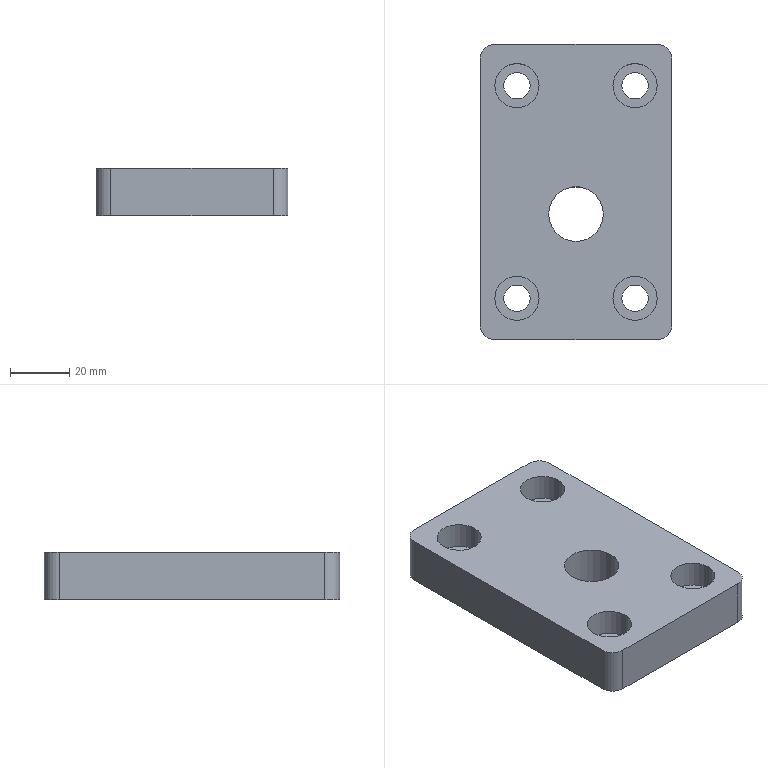Part | NX | features BREP 1 | 1 solid | 32 faces | box 65 x 100 x 16 mm | volume 91213 mm3 | cylinder 22 | plane 10 | commonest cylinder face diameters 9 x8 15 x8 10 x4 18.5 x2
STEP:
#1=CARTESIAN_POINT('',(-9.25,-7.5,0.));
#2=VERTEX_POINT('',#1);
#3=CARTESIAN_POINT('',(9.25,-7.5,0.));
#4=VERTEX_POINT('',#3);
#5=CARTESIAN_POINT('',(0.,-7.5,0.));
#6=DIRECTION('',(0.,0.,1.));
#7=DIRECTION('',(1.,0.,0.));
#8=AXIS2_PLACEMENT_3D('',#5,#6,#7);
#9=CIRCLE('',#8,9.25);
#10=EDGE_CURVE('',#2,#4,#9,.T.);
#11=ORIENTED_EDGE('',*,*,#10,.F.);
#12=CARTESIAN_POINT('',(-9.25,-7.5,16.));
#13=VERTEX_POINT('',#12);
#14=CARTESIAN_POINT('',(-9.25,-7.5,16.));
#15=DIRECTION('',(0.,0.,1.));
#16=VECTOR('',#15,1000.);
#17=LINE('',#14,#16);
#18=EDGE_CURVE('',#13,#2,#17,.F.);
#19=ORIENTED_EDGE('',*,*,#18,.F.);
#20=CARTESIAN_POINT('',(9.25,-7.5,16.));
#21=VERTEX_POINT('',#20);
#22=CARTESIAN_POINT('',(0.,-7.5,16.));
#23=DIRECTION('',(0.,0.,1.));
#24=DIRECTION('',(1.,0.,0.));
#25=AXIS2_PLACEMENT_3D('',#22,#23,#24);
#26=CIRCLE('',#25,9.25);
#27=EDGE_CURVE('',#13,#21,#26,.T.);
#28=ORIENTED_EDGE('',*,*,#27,.T.);
#29=CARTESIAN_POINT('',(9.25,-7.5,16.));
#30=DIRECTION('',(0.,0.,1.));
#31=VECTOR('',#30,1000.);
#32=LINE('',#29,#31);
#33=EDGE_CURVE('',#21,#4,#32,.F.);
#34=ORIENTED_EDGE('',*,*,#33,.T.);
#35=EDGE_LOOP('',(#11,#19,#28,#34));
#36=FACE_BOUND('',#35,.T.);
#37=CARTESIAN_POINT('',(0.,-7.5,16.));
#38=DIRECTION('',(0.,0.,1.));
#39=DIRECTION('',(1.,0.,0.));
#40=AXIS2_PLACEMENT_3D('',#37,#38,#39);
#41=CYLINDRICAL_SURFACE('',#40,9.25);
#42=ADVANCED_FACE('',(#36),#41,.F.);
#43=CARTESIAN_POINT('',(-27.5,36.,7.));
#44=VERTEX_POINT('',#43);
#45=CARTESIAN_POINT('',(-12.5,36.,7.));
#46=VERTEX_POINT('',#45);
#47=CARTESIAN_POINT('',(-20.,36.,7.));
#48=DIRECTION('',(0.,0.,1.));
#49=DIRECTION('',(1.,0.,0.));
#50=AXIS2_PLACEMENT_3D('',#47,#48,#49);
#51=CIRCLE('',#50,7.5);
#52=EDGE_CURVE('',#44,#46,#51,.T.);
#53=ORIENTED_EDGE('',*,*,#52,.F.);
#54=CARTESIAN_POINT('',(-27.5,36.,16.));
#55=VERTEX_POINT('',#54);
#56=CARTESIAN_POINT('',(-27.5,36.,16.));
#57=DIRECTION('',(0.,0.,1.));
#58=VECTOR('',#57,1000.);
#59=LINE('',#56,#58);
#60=EDGE_CURVE('',#55,#44,#59,.F.);
#61=ORIENTED_EDGE('',*,*,#60,.F.);
#62=CARTESIAN_POINT('',(-12.5,36.,16.));
#63=VERTEX_POINT('',#62);
#64=CARTESIAN_POINT('',(-20.,36.,16.));
#65=DIRECTION('',(0.,0.,1.));
#66=DIRECTION('',(1.,0.,0.));
#67=AXIS2_PLACEMENT_3D('',#64,#65,#66);
#68=CIRCLE('',#67,7.5);
#69=EDGE_CURVE('',#55,#63,#68,.T.);
#70=ORIENTED_EDGE('',*,*,#69,.T.);
#71=CARTESIAN_POINT('',(-12.5,36.,16.));
#72=DIRECTION('',(0.,0.,1.));
#73=VECTOR('',#72,1000.);
#74=LINE('',#71,#73);
#75=EDGE_CURVE('',#63,#46,#74,.F.);
#76=ORIENTED_EDGE('',*,*,#75,.T.);
#77=EDGE_LOOP('',(#53,#61,#70,#76));
#78=FACE_BOUND('',#77,.T.);
#79=CARTESIAN_POINT('',(-20.,36.,16.));
#80=DIRECTION('',(0.,0.,1.));
#81=DIRECTION('',(1.,0.,0.));
#82=AXIS2_PLACEMENT_3D('',#79,#80,#81);
#83=CYLINDRICAL_SURFACE('',#82,7.5);
#84=ADVANCED_FACE('',(#78),#83,.F.);
#85=CARTESIAN_POINT('',(-24.5,36.,0.));
#86=VERTEX_POINT('',#85);
#87=CARTESIAN_POINT('',(-15.5,36.,0.));
#88=VERTEX_POINT('',#87);
#89=CARTESIAN_POINT('',(-20.,36.,0.));
#90=DIRECTION('',(0.,0.,1.));
#91=DIRECTION('',(1.,0.,0.));
#92=AXIS2_PLACEMENT_3D('',#89,#90,#91);
#93=CIRCLE('',#92,4.5);
#94=EDGE_CURVE('',#86,#88,#93,.T.);
#95=ORIENTED_EDGE('',*,*,#94,.F.);
#96=CARTESIAN_POINT('',(-24.5,36.,7.));
#97=VERTEX_POINT('',#96);
#98=CARTESIAN_POINT('',(-24.5,36.,16.));
#99=DIRECTION('',(0.,0.,1.));
#100=VECTOR('',#99,1000.);
#101=LINE('',#98,#100);
#102=EDGE_CURVE('',#97,#86,#101,.F.);
#103=ORIENTED_EDGE('',*,*,#102,.F.);
#104=CARTESIAN_POINT('',(-15.5,36.,7.));
#105=VERTEX_POINT('',#104);
#106=CARTESIAN_POINT('',(-20.,36.,7.));
#107=DIRECTION('',(0.,0.,1.));
#108=DIRECTION('',(1.,0.,0.));
#109=AXIS2_PLACEMENT_3D('',#106,#107,#108);
#110=CIRCLE('',#109,4.5);
#111=EDGE_CURVE('',#97,#105,#110,.T.);
#112=ORIENTED_EDGE('',*,*,#111,.T.);
#113=CARTESIAN_POINT('',(-15.5,36.,16.));
#114=DIRECTION('',(0.,0.,1.));
#115=VECTOR('',#114,1000.);
#116=LINE('',#113,#115);
#117=EDGE_CURVE('',#105,#88,#116,.F.);
#118=ORIENTED_EDGE('',*,*,#117,.T.);
#119=EDGE_LOOP('',(#95,#103,#112,#118));
#120=FACE_BOUND('',#119,.T.);
#121=CARTESIAN_POINT('',(-20.,36.,16.));
#122=DIRECTION('',(0.,0.,1.));
#123=DIRECTION('',(1.,0.,0.));
#124=AXIS2_PLACEMENT_3D('',#121,#122,#123);
#125=CYLINDRICAL_SURFACE('',#124,4.5);
#126=ADVANCED_FACE('',(#120),#125,.F.);
#127=CARTESIAN_POINT('',(12.5,36.,7.));
#128=VERTEX_POINT('',#127);
#129=CARTESIAN_POINT('',(27.5,36.,7.));
#130=VERTEX_POINT('',#129);
#131=CARTESIAN_POINT('',(20.,36.,7.));
#132=DIRECTION('',(0.,0.,1.));
#133=DIRECTION('',(1.,0.,0.));
#134=AXIS2_PLACEMENT_3D('',#131,#132,#133);
#135=CIRCLE('',#134,7.5);
#136=EDGE_CURVE('',#128,#130,#135,.T.);
#137=ORIENTED_EDGE('',*,*,#136,.F.);
#138=CARTESIAN_POINT('',(12.5,36.,16.));
#139=VERTEX_POINT('',#138);
#140=CARTESIAN_POINT('',(12.5,36.,16.));
#141=DIRECTION('',(0.,0.,1.));
#142=VECTOR('',#141,1000.);
#143=LINE('',#140,#142);
#144=EDGE_CURVE('',#139,#128,#143,.F.);
#145=ORIENTED_EDGE('',*,*,#144,.F.);
#146=CARTESIAN_POINT('',(27.5,36.,16.));
#147=VERTEX_POINT('',#146);
#148=CARTESIAN_POINT('',(20.,36.,16.));
#149=DIRECTION('',(0.,0.,1.));
#150=DIRECTION('',(1.,0.,0.));
#151=AXIS2_PLACEMENT_3D('',#148,#149,#150);
#152=CIRCLE('',#151,7.5);
#153=EDGE_CURVE('',#139,#147,#152,.T.);
#154=ORIENTED_EDGE('',*,*,#153,.T.);
#155=CARTESIAN_POINT('',(27.5,36.,16.));
#156=DIRECTION('',(0.,0.,1.));
#157=VECTOR('',#156,1000.);
#158=LINE('',#155,#157);
#159=EDGE_CURVE('',#147,#130,#158,.F.);
#160=ORIENTED_EDGE('',*,*,#159,.T.);
#161=EDGE_LOOP('',(#137,#145,#154,#160));
#162=FACE_BOUND('',#161,.T.);
#163=CARTESIAN_POINT('',(20.,36.,16.));
#164=DIRECTION('',(0.,0.,1.));
#165=DIRECTION('',(1.,0.,0.));
#166=AXIS2_PLACEMENT_3D('',#163,#164,#165);
#167=CYLINDRICAL_SURFACE('',#166,7.5);
#168=ADVANCED_FACE('',(#162),#167,.F.);
#169=CARTESIAN_POINT('',(15.5,36.,0.));
#170=VERTEX_POINT('',#169);
#171=CARTESIAN_POINT('',(24.5,36.,0.));
#172=VERTEX_POINT('',#171);
#173=CARTESIAN_POINT('',(20.,36.,0.));
#174=DIRECTION('',(0.,0.,1.));
#175=DIRECTION('',(1.,0.,0.));
#176=AXIS2_PLACEMENT_3D('',#173,#174,#175);
#177=CIRCLE('',#176,4.5);
#178=EDGE_CURVE('',#170,#172,#177,.T.);
#179=ORIENTED_EDGE('',*,*,#178,.F.);
#180=CARTESIAN_POINT('',(15.5,36.,7.));
#181=VERTEX_POINT('',#180);
#182=CARTESIAN_POINT('',(15.5,36.,16.));
#183=DIRECTION('',(0.,0.,1.));
#184=VECTOR('',#183,1000.);
#185=LINE('',#182,#184);
#186=EDGE_CURVE('',#181,#170,#185,.F.);
#187=ORIENTED_EDGE('',*,*,#186,.F.);
#188=CARTESIAN_POINT('',(24.5,36.,7.));
#189=VERTEX_POINT('',#188);
#190=CARTESIAN_POINT('',(20.,36.,7.));
#191=DIRECTION('',(0.,0.,1.));
#192=DIRECTION('',(1.,0.,0.));
#193=AXIS2_PLACEMENT_3D('',#190,#191,#192);
#194=CIRCLE('',#193,4.5);
#195=EDGE_CURVE('',#181,#189,#194,.T.);
#196=ORIENTED_EDGE('',*,*,#195,.T.);
#197=CARTESIAN_POINT('',(24.5,36.,16.));
#198=DIRECTION('',(0.,0.,1.));
#199=VECTOR('',#198,1000.);
#200=LINE('',#197,#199);
#201=EDGE_CURVE('',#189,#172,#200,.F.);
#202=ORIENTED_EDGE('',*,*,#201,.T.);
#203=EDGE_LOOP('',(#179,#187,#196,#202));
#204=FACE_BOUND('',#203,.T.);
#205=CARTESIAN_POINT('',(20.,36.,16.));
#206=DIRECTION('',(0.,0.,1.));
#207=DIRECTION('',(1.,0.,0.));
#208=AXIS2_PLACEMENT_3D('',#205,#206,#207);
#209=CYLINDRICAL_SURFACE('',#208,4.5);
#210=ADVANCED_FACE('',(#204),#209,.F.);
#211=CARTESIAN_POINT('',(-27.5,-36.,7.));
#212=VERTEX_POINT('',#211);
#213=CARTESIAN_POINT('',(-12.5,-36.,7.));
#214=VERTEX_POINT('',#213);
#215=CARTESIAN_POINT('',(-20.,-36.,7.));
#216=DIRECTION('',(0.,0.,1.));
#217=DIRECTION('',(1.,0.,0.));
#218=AXIS2_PLACEMENT_3D('',#215,#216,#217);
#219=CIRCLE('',#218,7.5);
#220=EDGE_CURVE('',#212,#214,#219,.T.);
#221=ORIENTED_EDGE('',*,*,#220,.F.);
#222=CARTESIAN_POINT('',(-27.5,-36.,16.));
#223=VERTEX_POINT('',#222);
#224=CARTESIAN_POINT('',(-27.5,-36.,16.));
#225=DIRECTION('',(0.,0.,1.));
#226=VECTOR('',#225,1000.);
#227=LINE('',#224,#226);
#228=EDGE_CURVE('',#223,#212,#227,.F.);
#229=ORIENTED_EDGE('',*,*,#228,.F.);
#230=CARTESIAN_POINT('',(-12.5,-36.,16.));
#231=VERTEX_POINT('',#230);
#232=CARTESIAN_POINT('',(-20.,-36.,16.));
#233=DIRECTION('',(0.,0.,1.));
#234=DIRECTION('',(1.,0.,0.));
#235=AXIS2_PLACEMENT_3D('',#232,#233,#234);
#236=CIRCLE('',#235,7.5);
#237=EDGE_CURVE('',#223,#231,#236,.T.);
#238=ORIENTED_EDGE('',*,*,#237,.T.);
#239=CARTESIAN_POINT('',(-12.5,-36.,16.));
#240=DIRECTION('',(0.,0.,1.));
#241=VECTOR('',#240,1000.);
#242=LINE('',#239,#241);
#243=EDGE_CURVE('',#231,#214,#242,.F.);
#244=ORIENTED_EDGE('',*,*,#243,.T.);
#245=EDGE_LOOP('',(#221,#229,#238,#244));
#246=FACE_BOUND('',#245,.T.);
#247=CARTESIAN_POINT('',(-20.,-36.,16.));
#248=DIRECTION('',(0.,0.,1.));
#249=DIRECTION('',(1.,0.,0.));
#250=AXIS2_PLACEMENT_3D('',#247,#248,#249);
#251=CYLINDRICAL_SURFACE('',#250,7.5);
#252=ADVANCED_FACE('',(#246),#251,.F.);
#253=CARTESIAN_POINT('',(-24.5,-36.,0.));
#254=VERTEX_POINT('',#253);
#255=CARTESIAN_POINT('',(-15.5,-36.,0.));
#256=VERTEX_POINT('',#255);
#257=CARTESIAN_POINT('',(-20.,-36.,0.));
#258=DIRECTION('',(0.,0.,1.));
#259=DIRECTION('',(1.,0.,0.));
#260=AXIS2_PLACEMENT_3D('',#257,#258,#259);
#261=CIRCLE('',#260,4.5);
#262=EDGE_CURVE('',#254,#256,#261,.T.);
#263=ORIENTED_EDGE('',*,*,#262,.F.);
#264=CARTESIAN_POINT('',(-24.5,-36.,7.));
#265=VERTEX_POINT('',#264);
#266=CARTESIAN_POINT('',(-24.5,-36.,16.));
#267=DIRECTION('',(0.,0.,1.));
#268=VECTOR('',#267,1000.);
#269=LINE('',#266,#268);
#270=EDGE_CURVE('',#265,#254,#269,.F.);
#271=ORIENTED_EDGE('',*,*,#270,.F.);
#272=CARTESIAN_POINT('',(-15.5,-36.,7.));
#273=VERTEX_POINT('',#272);
#274=CARTESIAN_POINT('',(-20.,-36.,7.));
#275=DIRECTION('',(0.,0.,1.));
#276=DIRECTION('',(1.,0.,0.));
#277=AXIS2_PLACEMENT_3D('',#274,#275,#276);
#278=CIRCLE('',#277,4.5);
#279=EDGE_CURVE('',#265,#273,#278,.T.);
#280=ORIENTED_EDGE('',*,*,#279,.T.);
#281=CARTESIAN_POINT('',(-15.5,-36.,16.));
#282=DIRECTION('',(0.,0.,1.));
#283=VECTOR('',#282,1000.);
#284=LINE('',#281,#283);
#285=EDGE_CURVE('',#273,#256,#284,.F.);
#286=ORIENTED_EDGE('',*,*,#285,.T.);
#287=EDGE_LOOP('',(#263,#271,#280,#286));
#288=FACE_BOUND('',#287,.T.);
#289=CARTESIAN_POINT('',(-20.,-36.,16.));
#290=DIRECTION('',(0.,0.,1.));
#291=DIRECTION('',(1.,0.,0.));
#292=AXIS2_PLACEMENT_3D('',#289,#290,#291);
#293=CYLINDRICAL_SURFACE('',#292,4.5);
#294=ADVANCED_FACE('',(#288),#293,.F.);
#295=CARTESIAN_POINT('',(12.5,-36.,7.));
#296=VERTEX_POINT('',#295);
#297=CARTESIAN_POINT('',(27.5,-36.,7.));
#298=VERTEX_POINT('',#297);
#299=CARTESIAN_POINT('',(20.,-36.,7.));
#300=DIRECTION('',(0.,0.,1.));
#301=DIRECTION('',(1.,0.,0.));
#302=AXIS2_PLACEMENT_3D('',#299,#300,#301);
#303=CIRCLE('',#302,7.5);
#304=EDGE_CURVE('',#296,#298,#303,.T.);
#305=ORIENTED_EDGE('',*,*,#304,.F.);
#306=CARTESIAN_POINT('',(12.5,-36.,16.));
#307=VERTEX_POINT('',#306);
#308=CARTESIAN_POINT('',(12.5,-36.,16.));
#309=DIRECTION('',(0.,0.,1.));
#310=VECTOR('',#309,1000.);
#311=LINE('',#308,#310);
#312=EDGE_CURVE('',#307,#296,#311,.F.);
#313=ORIENTED_EDGE('',*,*,#312,.F.);
#314=CARTESIAN_POINT('',(27.5,-36.,16.));
#315=VERTEX_POINT('',#314);
#316=CARTESIAN_POINT('',(20.,-36.,16.));
#317=DIRECTION('',(0.,0.,1.));
#318=DIRECTION('',(1.,0.,0.));
#319=AXIS2_PLACEMENT_3D('',#316,#317,#318);
#320=CIRCLE('',#319,7.5);
#321=EDGE_CURVE('',#307,#315,#320,.T.);
#322=ORIENTED_EDGE('',*,*,#321,.T.);
#323=CARTESIAN_POINT('',(27.5,-36.,16.));
#324=DIRECTION('',(0.,0.,1.));
#325=VECTOR('',#324,1000.);
#326=LINE('',#323,#325);
#327=EDGE_CURVE('',#315,#298,#326,.F.);
#328=ORIENTED_EDGE('',*,*,#327,.T.);
#329=EDGE_LOOP('',(#305,#313,#322,#328));
#330=FACE_BOUND('',#329,.T.);
#331=CARTESIAN_POINT('',(20.,-36.,16.));
#332=DIRECTION('',(0.,0.,1.));
#333=DIRECTION('',(1.,0.,0.));
#334=AXIS2_PLACEMENT_3D('',#331,#332,#333);
#335=CYLINDRICAL_SURFACE('',#334,7.5);
#336=ADVANCED_FACE('',(#330),#335,.F.);
#337=CARTESIAN_POINT('',(15.5,-36.,0.));
#338=VERTEX_POINT('',#337);
#339=CARTESIAN_POINT('',(24.5,-36.,0.));
#340=VERTEX_POINT('',#339);
#341=CARTESIAN_POINT('',(20.,-36.,0.));
#342=DIRECTION('',(0.,0.,1.));
#343=DIRECTION('',(1.,0.,0.));
#344=AXIS2_PLACEMENT_3D('',#341,#342,#343);
#345=CIRCLE('',#344,4.5);
#346=EDGE_CURVE('',#338,#340,#345,.T.);
#347=ORIENTED_EDGE('',*,*,#346,.F.);
#348=CARTESIAN_POINT('',(15.5,-36.,7.));
#349=VERTEX_POINT('',#348);
#350=CARTESIAN_POINT('',(15.5,-36.,16.));
#351=DIRECTION('',(0.,0.,1.));
#352=VECTOR('',#351,1000.);
#353=LINE('',#350,#352);
#354=EDGE_CURVE('',#349,#338,#353,.F.);
#355=ORIENTED_EDGE('',*,*,#354,.F.);
#356=CARTESIAN_POINT('',(24.5,-36.,7.));
#357=VERTEX_POINT('',#356);
#358=CARTESIAN_POINT('',(20.,-36.,7.));
#359=DIRECTION('',(0.,0.,1.));
#360=DIRECTION('',(1.,0.,0.));
#361=AXIS2_PLACEMENT_3D('',#358,#359,#360);
#362=CIRCLE('',#361,4.5);
#363=EDGE_CURVE('',#349,#357,#362,.T.);
#364=ORIENTED_EDGE('',*,*,#363,.T.);
#365=CARTESIAN_POINT('',(24.5,-36.,16.));
#366=DIRECTION('',(0.,0.,1.));
#367=VECTOR('',#366,1000.);
#368=LINE('',#365,#367);
#369=EDGE_CURVE('',#357,#340,#368,.F.);
#370=ORIENTED_EDGE('',*,*,#369,.T.);
#371=EDGE_LOOP('',(#347,#355,#364,#370));
#372=FACE_BOUND('',#371,.T.);
#373=CARTESIAN_POINT('',(20.,-36.,16.));
#374=DIRECTION('',(0.,0.,1.));
#375=DIRECTION('',(1.,0.,0.));
#376=AXIS2_PLACEMENT_3D('',#373,#374,#375);
#377=CYLINDRICAL_SURFACE('',#376,4.5);
#378=ADVANCED_FACE('',(#372),#377,.F.);
#379=CARTESIAN_POINT('',(32.5,-45.,0.));
#380=VERTEX_POINT('',#379);
#381=CARTESIAN_POINT('',(32.5,45.,0.));
#382=VERTEX_POINT('',#381);
#383=CARTESIAN_POINT('',(32.5,-50.,0.));
#384=DIRECTION('',(0.,1.,0.));
#385=VECTOR('',#384,1000.);
#386=LINE('',#383,#385);
#387=EDGE_CURVE('',#380,#382,#386,.T.);
#388=ORIENTED_EDGE('',*,*,#387,.T.);
#389=CARTESIAN_POINT('',(32.5,45.,16.));
#390=VERTEX_POINT('',#389);
#391=CARTESIAN_POINT('',(32.5,45.,16.));
#392=DIRECTION('',(0.,0.,1.));
#393=VECTOR('',#392,1000.);
#394=LINE('',#391,#393);
#395=EDGE_CURVE('',#382,#390,#394,.T.);
#396=ORIENTED_EDGE('',*,*,#395,.T.);
#397=CARTESIAN_POINT('',(32.5,-45.,16.));
#398=VERTEX_POINT('',#397);
#399=CARTESIAN_POINT('',(32.5,-50.,16.));
#400=DIRECTION('',(0.,1.,0.));
#401=VECTOR('',#400,1000.);
#402=LINE('',#399,#401);
#403=EDGE_CURVE('',#398,#390,#402,.T.);
#404=ORIENTED_EDGE('',*,*,#403,.F.);
#405=CARTESIAN_POINT('',(32.5,-45.,16.));
#406=DIRECTION('',(0.,0.,-1.));
#407=VECTOR('',#406,1000.);
#408=LINE('',#405,#407);
#409=EDGE_CURVE('',#398,#380,#408,.T.);
#410=ORIENTED_EDGE('',*,*,#409,.T.);
#411=EDGE_LOOP('',(#388,#396,#404,#410));
#412=FACE_BOUND('',#411,.T.);
#413=CARTESIAN_POINT('',(32.5,-50.,16.));
#414=DIRECTION('',(-1.,0.,0.));
#415=DIRECTION('',(0.,0.,1.));
#416=AXIS2_PLACEMENT_3D('',#413,#414,#415);
#417=PLANE('',#416);
#418=ADVANCED_FACE('',(#412),#417,.F.);
#419=CARTESIAN_POINT('',(27.5,50.,16.));
#420=VERTEX_POINT('',#419);
#421=CARTESIAN_POINT('',(-27.5,50.,16.));
#422=VERTEX_POINT('',#421);
#423=CARTESIAN_POINT('',(-32.5,50.,16.));
#424=DIRECTION('',(-1.,0.,0.));
#425=VECTOR('',#424,1000.);
#426=LINE('',#423,#425);
#427=EDGE_CURVE('',#420,#422,#426,.T.);
#428=ORIENTED_EDGE('',*,*,#427,.F.);
#429=CARTESIAN_POINT('',(27.5,50.,0.));
#430=VERTEX_POINT('',#429);
#431=CARTESIAN_POINT('',(27.5,50.,16.));
#432=DIRECTION('',(0.,0.,-1.));
#433=VECTOR('',#432,1000.);
#434=LINE('',#431,#433);
#435=EDGE_CURVE('',#420,#430,#434,.T.);
#436=ORIENTED_EDGE('',*,*,#435,.T.);
#437=CARTESIAN_POINT('',(-27.5,50.,0.));
#438=VERTEX_POINT('',#437);
#439=CARTESIAN_POINT('',(-32.5,50.,0.));
#440=DIRECTION('',(-1.,0.,0.));
#441=VECTOR('',#440,1000.);
#442=LINE('',#439,#441);
#443=EDGE_CURVE('',#430,#438,#442,.T.);
#444=ORIENTED_EDGE('',*,*,#443,.T.);
#445=CARTESIAN_POINT('',(-27.5,50.,16.));
#446=DIRECTION('',(0.,0.,1.));
#447=VECTOR('',#446,1000.);
#448=LINE('',#445,#447);
#449=EDGE_CURVE('',#438,#422,#448,.T.);
#450=ORIENTED_EDGE('',*,*,#449,.T.);
#451=EDGE_LOOP('',(#428,#436,#444,#450));
#452=FACE_BOUND('',#451,.T.);
#453=CARTESIAN_POINT('',(-32.5,50.,16.));
#454=DIRECTION('',(0.,-1.,0.));
#455=DIRECTION('',(0.,0.,-1.));
#456=AXIS2_PLACEMENT_3D('',#453,#454,#455);
#457=PLANE('',#456);
#458=ADVANCED_FACE('',(#452),#457,.F.);
#459=CARTESIAN_POINT('',(-32.5,45.,0.));
#460=VERTEX_POINT('',#459);
#461=CARTESIAN_POINT('',(-32.5,-45.,0.));
#462=VERTEX_POINT('',#461);
#463=CARTESIAN_POINT('',(-32.5,-50.,0.));
#464=DIRECTION('',(0.,-1.,0.));
#465=VECTOR('',#464,1000.);
#466=LINE('',#463,#465);
#467=EDGE_CURVE('',#460,#462,#466,.T.);
#468=ORIENTED_EDGE('',*,*,#467,.T.);
#469=CARTESIAN_POINT('',(-32.5,-45.,16.));
#470=VERTEX_POINT('',#469);
#471=CARTESIAN_POINT('',(-32.5,-45.,16.));
#472=DIRECTION('',(0.,0.,1.));
#473=VECTOR('',#472,1000.);
#474=LINE('',#471,#473);
#475=EDGE_CURVE('',#462,#470,#474,.T.);
#476=ORIENTED_EDGE('',*,*,#475,.T.);
#477=CARTESIAN_POINT('',(-32.5,45.,16.));
#478=VERTEX_POINT('',#477);
#479=CARTESIAN_POINT('',(-32.5,-50.,16.));
#480=DIRECTION('',(0.,-1.,0.));
#481=VECTOR('',#480,1000.);
#482=LINE('',#479,#481);
#483=EDGE_CURVE('',#478,#470,#482,.T.);
#484=ORIENTED_EDGE('',*,*,#483,.F.);
#485=CARTESIAN_POINT('',(-32.5,45.,16.));
#486=DIRECTION('',(0.,0.,-1.));
#487=VECTOR('',#486,1000.);
#488=LINE('',#485,#487);
#489=EDGE_CURVE('',#478,#460,#488,.T.);
#490=ORIENTED_EDGE('',*,*,#489,.T.);
#491=EDGE_LOOP('',(#468,#476,#484,#490));
#492=FACE_BOUND('',#491,.T.);
#493=CARTESIAN_POINT('',(-32.5,-50.,16.));
#494=DIRECTION('',(1.,0.,0.));
#495=DIRECTION('',(0.,1.,0.));
#496=AXIS2_PLACEMENT_3D('',#493,#494,#495);
#497=PLANE('',#496);
#498=ADVANCED_FACE('',(#492),#497,.F.);
#499=CARTESIAN_POINT('',(-27.5,-50.,0.));
#500=VERTEX_POINT('',#499);
#501=CARTESIAN_POINT('',(27.5,-50.,0.));
#502=VERTEX_POINT('',#501);
#503=CARTESIAN_POINT('',(-32.5,-50.,0.));
#504=DIRECTION('',(1.,0.,0.));
#505=VECTOR('',#504,1000.);
#506=LINE('',#503,#505);
#507=EDGE_CURVE('',#500,#502,#506,.T.);
#508=ORIENTED_EDGE('',*,*,#507,.T.);
#509=CARTESIAN_POINT('',(27.5,-50.,16.));
#510=VERTEX_POINT('',#509);
#511=CARTESIAN_POINT('',(27.5,-50.,16.));
#512=DIRECTION('',(0.,0.,1.));
#513=VECTOR('',#512,1000.);
#514=LINE('',#511,#513);
#515=EDGE_CURVE('',#502,#510,#514,.T.);
#516=ORIENTED_EDGE('',*,*,#515,.T.);
#517=CARTESIAN_POINT('',(-27.5,-50.,16.));
#518=VERTEX_POINT('',#517);
#519=CARTESIAN_POINT('',(-32.5,-50.,16.));
#520=DIRECTION('',(1.,0.,0.));
#521=VECTOR('',#520,1000.);
#522=LINE('',#519,#521);
#523=EDGE_CURVE('',#518,#510,#522,.T.);
#524=ORIENTED_EDGE('',*,*,#523,.F.);
#525=CARTESIAN_POINT('',(-27.5,-50.,16.));
#526=DIRECTION('',(0.,0.,-1.));
#527=VECTOR('',#526,1000.);
#528=LINE('',#525,#527);
#529=EDGE_CURVE('',#518,#500,#528,.T.);
#530=ORIENTED_EDGE('',*,*,#529,.T.);
#531=EDGE_LOOP('',(#508,#516,#524,#530));
#532=FACE_BOUND('',#531,.T.);
#533=CARTESIAN_POINT('',(-32.5,-50.,16.));
#534=DIRECTION('',(0.,1.,0.));
#535=DIRECTION('',(1.,0.,0.));
#536=AXIS2_PLACEMENT_3D('',#533,#534,#535);
#537=PLANE('',#536);
#538=ADVANCED_FACE('',(#532),#537,.F.);
#539=ORIENTED_EDGE('',*,*,#403,.T.);
#540=CARTESIAN_POINT('',(27.5,45.,16.));
#541=DIRECTION('',(0.,0.,1.));
#542=DIRECTION('',(-1.,0.,0.));
#543=AXIS2_PLACEMENT_3D('',#540,#541,#542);
#544=CIRCLE('',#543,5.);
#545=EDGE_CURVE('',#390,#420,#544,.T.);
#546=ORIENTED_EDGE('',*,*,#545,.T.);
#547=ORIENTED_EDGE('',*,*,#427,.T.);
#548=CARTESIAN_POINT('',(-27.5,45.,16.));
#549=DIRECTION('',(0.,0.,1.));
#550=DIRECTION('',(-1.,0.,0.));
#551=AXIS2_PLACEMENT_3D('',#548,#549,#550);
#552=CIRCLE('',#551,5.);
#553=EDGE_CURVE('',#422,#478,#552,.T.);
#554=ORIENTED_EDGE('',*,*,#553,.T.);
#555=ORIENTED_EDGE('',*,*,#483,.T.);
#556=CARTESIAN_POINT('',(-27.5,-45.,16.));
#557=DIRECTION('',(0.,0.,1.));
#558=DIRECTION('',(-1.,0.,0.));
#559=AXIS2_PLACEMENT_3D('',#556,#557,#558);
#560=CIRCLE('',#559,5.);
#561=EDGE_CURVE('',#470,#518,#560,.T.);
#562=ORIENTED_EDGE('',*,*,#561,.T.);
#563=ORIENTED_EDGE('',*,*,#523,.T.);
#564=CARTESIAN_POINT('',(27.5,-45.,16.));
#565=DIRECTION('',(0.,0.,1.));
#566=DIRECTION('',(-1.,0.,0.));
#567=AXIS2_PLACEMENT_3D('',#564,#565,#566);
#568=CIRCLE('',#567,5.);
#569=EDGE_CURVE('',#510,#398,#568,.T.);
#570=ORIENTED_EDGE('',*,*,#569,.T.);
#571=EDGE_LOOP('',(#539,#546,#547,#554,#555,#562,#563,#570));
#572=FACE_BOUND('',#571,.T.);
#573=CARTESIAN_POINT('',(0.,-7.5,16.));
#574=DIRECTION('',(0.,0.,1.));
#575=DIRECTION('',(1.,0.,0.));
#576=AXIS2_PLACEMENT_3D('',#573,#574,#575);
#577=CIRCLE('',#576,9.25);
#578=EDGE_CURVE('',#21,#13,#577,.T.);
#579=ORIENTED_EDGE('',*,*,#578,.F.);
#580=ORIENTED_EDGE('',*,*,#27,.F.);
#581=EDGE_LOOP('',(#579,#580));
#582=FACE_BOUND('',#581,.T.);
#583=CARTESIAN_POINT('',(-20.,36.,16.));
#584=DIRECTION('',(0.,0.,1.));
#585=DIRECTION('',(1.,0.,0.));
#586=AXIS2_PLACEMENT_3D('',#583,#584,#585);
#587=CIRCLE('',#586,7.5);
#588=EDGE_CURVE('',#63,#55,#587,.T.);
#589=ORIENTED_EDGE('',*,*,#588,.F.);
#590=ORIENTED_EDGE('',*,*,#69,.F.);
#591=EDGE_LOOP('',(#589,#590));
#592=FACE_BOUND('',#591,.T.);
#593=CARTESIAN_POINT('',(20.,36.,16.));
#594=DIRECTION('',(0.,0.,1.));
#595=DIRECTION('',(1.,0.,0.));
#596=AXIS2_PLACEMENT_3D('',#593,#594,#595);
#597=CIRCLE('',#596,7.5);
#598=EDGE_CURVE('',#147,#139,#597,.T.);
#599=ORIENTED_EDGE('',*,*,#598,.F.);
#600=ORIENTED_EDGE('',*,*,#153,.F.);
#601=EDGE_LOOP('',(#599,#600));
#602=FACE_BOUND('',#601,.T.);
#603=CARTESIAN_POINT('',(-20.,-36.,16.));
#604=DIRECTION('',(0.,0.,1.));
#605=DIRECTION('',(1.,0.,0.));
#606=AXIS2_PLACEMENT_3D('',#603,#604,#605);
#607=CIRCLE('',#606,7.5);
#608=EDGE_CURVE('',#231,#223,#607,.T.);
#609=ORIENTED_EDGE('',*,*,#608,.F.);
#610=ORIENTED_EDGE('',*,*,#237,.F.);
#611=EDGE_LOOP('',(#609,#610));
#612=FACE_BOUND('',#611,.T.);
#613=CARTESIAN_POINT('',(20.,-36.,16.));
#614=DIRECTION('',(0.,0.,1.));
#615=DIRECTION('',(1.,0.,0.));
#616=AXIS2_PLACEMENT_3D('',#613,#614,#615);
#617=CIRCLE('',#616,7.5);
#618=EDGE_CURVE('',#315,#307,#617,.T.);
#619=ORIENTED_EDGE('',*,*,#618,.F.);
#620=ORIENTED_EDGE('',*,*,#321,.F.);
#621=EDGE_LOOP('',(#619,#620));
#622=FACE_BOUND('',#621,.T.);
#623=CARTESIAN_POINT('',(0.,0.,16.));
#624=DIRECTION('',(0.,0.,-1.));
#625=DIRECTION('',(0.,-1.,0.));
#626=AXIS2_PLACEMENT_3D('',#623,#624,#625);
#627=PLANE('',#626);
#628=ADVANCED_FACE('',(#572,#582,#592,#602,#612,#622),#627,.F.);
#629=ORIENTED_EDGE('',*,*,#443,.F.);
#630=CARTESIAN_POINT('',(27.5,45.,0.));
#631=DIRECTION('',(0.,0.,-1.));
#632=DIRECTION('',(-1.,0.,0.));
#633=AXIS2_PLACEMENT_3D('',#630,#631,#632);
#634=CIRCLE('',#633,5.);
#635=EDGE_CURVE('',#430,#382,#634,.T.);
#636=ORIENTED_EDGE('',*,*,#635,.T.);
#637=ORIENTED_EDGE('',*,*,#387,.F.);
#638=CARTESIAN_POINT('',(27.5,-45.,0.));
#639=DIRECTION('',(0.,0.,-1.));
#640=DIRECTION('',(-1.,0.,0.));
#641=AXIS2_PLACEMENT_3D('',#638,#639,#640);
#642=CIRCLE('',#641,5.);
#643=EDGE_CURVE('',#380,#502,#642,.T.);
#644=ORIENTED_EDGE('',*,*,#643,.T.);
#645=ORIENTED_EDGE('',*,*,#507,.F.);
#646=CARTESIAN_POINT('',(-27.5,-45.,0.));
#647=DIRECTION('',(0.,0.,-1.));
#648=DIRECTION('',(-1.,0.,0.));
#649=AXIS2_PLACEMENT_3D('',#646,#647,#648);
#650=CIRCLE('',#649,5.);
#651=EDGE_CURVE('',#500,#462,#650,.T.);
#652=ORIENTED_EDGE('',*,*,#651,.T.);
#653=ORIENTED_EDGE('',*,*,#467,.F.);
#654=CARTESIAN_POINT('',(-27.5,45.,0.));
#655=DIRECTION('',(0.,0.,-1.));
#656=DIRECTION('',(-1.,0.,0.));
#657=AXIS2_PLACEMENT_3D('',#654,#655,#656);
#658=CIRCLE('',#657,5.);
#659=EDGE_CURVE('',#460,#438,#658,.T.);
#660=ORIENTED_EDGE('',*,*,#659,.T.);
#661=EDGE_LOOP('',(#629,#636,#637,#644,#645,#652,#653,#660));
#662=FACE_BOUND('',#661,.T.);
#663=CARTESIAN_POINT('',(0.,-7.5,0.));
#664=DIRECTION('',(0.,0.,1.));
#665=DIRECTION('',(1.,0.,0.));
#666=AXIS2_PLACEMENT_3D('',#663,#664,#665);
#667=CIRCLE('',#666,9.25);
#668=EDGE_CURVE('',#4,#2,#667,.T.);
#669=ORIENTED_EDGE('',*,*,#668,.T.);
#670=ORIENTED_EDGE('',*,*,#10,.T.);
#671=EDGE_LOOP('',(#669,#670));
#672=FACE_BOUND('',#671,.T.);
#673=CARTESIAN_POINT('',(-20.,36.,0.));
#674=DIRECTION('',(0.,0.,1.));
#675=DIRECTION('',(1.,0.,0.));
#676=AXIS2_PLACEMENT_3D('',#673,#674,#675);
#677=CIRCLE('',#676,4.5);
#678=EDGE_CURVE('',#88,#86,#677,.T.);
#679=ORIENTED_EDGE('',*,*,#678,.T.);
#680=ORIENTED_EDGE('',*,*,#94,.T.);
#681=EDGE_LOOP('',(#679,#680));
#682=FACE_BOUND('',#681,.T.);
#683=CARTESIAN_POINT('',(20.,36.,0.));
#684=DIRECTION('',(0.,0.,1.));
#685=DIRECTION('',(1.,0.,0.));
#686=AXIS2_PLACEMENT_3D('',#683,#684,#685);
#687=CIRCLE('',#686,4.5);
#688=EDGE_CURVE('',#172,#170,#687,.T.);
#689=ORIENTED_EDGE('',*,*,#688,.T.);
#690=ORIENTED_EDGE('',*,*,#178,.T.);
#691=EDGE_LOOP('',(#689,#690));
#692=FACE_BOUND('',#691,.T.);
#693=CARTESIAN_POINT('',(-20.,-36.,0.));
#694=DIRECTION('',(0.,0.,1.));
#695=DIRECTION('',(1.,0.,0.));
#696=AXIS2_PLACEMENT_3D('',#693,#694,#695);
#697=CIRCLE('',#696,4.5);
#698=EDGE_CURVE('',#256,#254,#697,.T.);
#699=ORIENTED_EDGE('',*,*,#698,.T.);
#700=ORIENTED_EDGE('',*,*,#262,.T.);
#701=EDGE_LOOP('',(#699,#700));
#702=FACE_BOUND('',#701,.T.);
#703=CARTESIAN_POINT('',(20.,-36.,0.));
#704=DIRECTION('',(0.,0.,1.));
#705=DIRECTION('',(1.,0.,0.));
#706=AXIS2_PLACEMENT_3D('',#703,#704,#705);
#707=CIRCLE('',#706,4.5);
#708=EDGE_CURVE('',#340,#338,#707,.T.);
#709=ORIENTED_EDGE('',*,*,#708,.T.);
#710=ORIENTED_EDGE('',*,*,#346,.T.);
#711=EDGE_LOOP('',(#709,#710));
#712=FACE_BOUND('',#711,.T.);
#713=CARTESIAN_POINT('',(0.,0.,0.));
#714=DIRECTION('',(0.,0.,-1.));
#715=DIRECTION('',(0.,-1.,0.));
#716=AXIS2_PLACEMENT_3D('',#713,#714,#715);
#717=PLANE('',#716);
#718=ADVANCED_FACE('',(#662,#672,#682,#692,#702,#712),#717,.T.);
#719=ORIENTED_EDGE('',*,*,#354,.T.);
#720=ORIENTED_EDGE('',*,*,#708,.F.);
#721=ORIENTED_EDGE('',*,*,#369,.F.);
#722=CARTESIAN_POINT('',(20.,-36.,7.));
#723=DIRECTION('',(0.,0.,1.));
#724=DIRECTION('',(1.,0.,0.));
#725=AXIS2_PLACEMENT_3D('',#722,#723,#724);
#726=CIRCLE('',#725,4.5);
#727=EDGE_CURVE('',#357,#349,#726,.T.);
#728=ORIENTED_EDGE('',*,*,#727,.T.);
#729=EDGE_LOOP('',(#719,#720,#721,#728));
#730=FACE_BOUND('',#729,.T.);
#731=CARTESIAN_POINT('',(20.,-36.,16.));
#732=DIRECTION('',(0.,0.,1.));
#733=DIRECTION('',(1.,0.,0.));
#734=AXIS2_PLACEMENT_3D('',#731,#732,#733);
#735=CYLINDRICAL_SURFACE('',#734,4.5);
#736=ADVANCED_FACE('',(#730),#735,.F.);
#737=CARTESIAN_POINT('',(20.,-36.,7.));
#738=DIRECTION('',(0.,0.,1.));
#739=DIRECTION('',(1.,0.,0.));
#740=AXIS2_PLACEMENT_3D('',#737,#738,#739);
#741=CIRCLE('',#740,7.5);
#742=EDGE_CURVE('',#298,#296,#741,.T.);
#743=ORIENTED_EDGE('',*,*,#742,.T.);
#744=ORIENTED_EDGE('',*,*,#304,.T.);
#745=EDGE_LOOP('',(#743,#744));
#746=FACE_BOUND('',#745,.T.);
#747=ORIENTED_EDGE('',*,*,#727,.F.);
#748=ORIENTED_EDGE('',*,*,#363,.F.);
#749=EDGE_LOOP('',(#747,#748));
#750=FACE_BOUND('',#749,.T.);
#751=CARTESIAN_POINT('',(24.5,-36.,7.));
#752=DIRECTION('',(0.,0.,-1.));
#753=DIRECTION('',(0.,-1.,0.));
#754=AXIS2_PLACEMENT_3D('',#751,#752,#753);
#755=PLANE('',#754);
#756=ADVANCED_FACE('',(#746,#750),#755,.F.);
#757=ORIENTED_EDGE('',*,*,#312,.T.);
#758=ORIENTED_EDGE('',*,*,#742,.F.);
#759=ORIENTED_EDGE('',*,*,#327,.F.);
#760=ORIENTED_EDGE('',*,*,#618,.T.);
#761=EDGE_LOOP('',(#757,#758,#759,#760));
#762=FACE_BOUND('',#761,.T.);
#763=CARTESIAN_POINT('',(20.,-36.,16.));
#764=DIRECTION('',(0.,0.,1.));
#765=DIRECTION('',(1.,0.,0.));
#766=AXIS2_PLACEMENT_3D('',#763,#764,#765);
#767=CYLINDRICAL_SURFACE('',#766,7.5);
#768=ADVANCED_FACE('',(#762),#767,.F.);
#769=ORIENTED_EDGE('',*,*,#270,.T.);
#770=ORIENTED_EDGE('',*,*,#698,.F.);
#771=ORIENTED_EDGE('',*,*,#285,.F.);
#772=CARTESIAN_POINT('',(-20.,-36.,7.));
#773=DIRECTION('',(0.,0.,1.));
#774=DIRECTION('',(1.,0.,0.));
#775=AXIS2_PLACEMENT_3D('',#772,#773,#774);
#776=CIRCLE('',#775,4.5);
#777=EDGE_CURVE('',#273,#265,#776,.T.);
#778=ORIENTED_EDGE('',*,*,#777,.T.);
#779=EDGE_LOOP('',(#769,#770,#771,#778));
#780=FACE_BOUND('',#779,.T.);
#781=CARTESIAN_POINT('',(-20.,-36.,16.));
#782=DIRECTION('',(0.,0.,1.));
#783=DIRECTION('',(1.,0.,0.));
#784=AXIS2_PLACEMENT_3D('',#781,#782,#783);
#785=CYLINDRICAL_SURFACE('',#784,4.5);
#786=ADVANCED_FACE('',(#780),#785,.F.);
#787=CARTESIAN_POINT('',(-20.,-36.,7.));
#788=DIRECTION('',(0.,0.,1.));
#789=DIRECTION('',(1.,0.,0.));
#790=AXIS2_PLACEMENT_3D('',#787,#788,#789);
#791=CIRCLE('',#790,7.5);
#792=EDGE_CURVE('',#214,#212,#791,.T.);
#793=ORIENTED_EDGE('',*,*,#792,.T.);
#794=ORIENTED_EDGE('',*,*,#220,.T.);
#795=EDGE_LOOP('',(#793,#794));
#796=FACE_BOUND('',#795,.T.);
#797=ORIENTED_EDGE('',*,*,#777,.F.);
#798=ORIENTED_EDGE('',*,*,#279,.F.);
#799=EDGE_LOOP('',(#797,#798));
#800=FACE_BOUND('',#799,.T.);
#801=CARTESIAN_POINT('',(-15.5,-36.,7.));
#802=DIRECTION('',(0.,0.,-1.));
#803=DIRECTION('',(0.,-1.,0.));
#804=AXIS2_PLACEMENT_3D('',#801,#802,#803);
#805=PLANE('',#804);
#806=ADVANCED_FACE('',(#796,#800),#805,.F.);
#807=ORIENTED_EDGE('',*,*,#228,.T.);
#808=ORIENTED_EDGE('',*,*,#792,.F.);
#809=ORIENTED_EDGE('',*,*,#243,.F.);
#810=ORIENTED_EDGE('',*,*,#608,.T.);
#811=EDGE_LOOP('',(#807,#808,#809,#810));
#812=FACE_BOUND('',#811,.T.);
#813=CARTESIAN_POINT('',(-20.,-36.,16.));
#814=DIRECTION('',(0.,0.,1.));
#815=DIRECTION('',(1.,0.,0.));
#816=AXIS2_PLACEMENT_3D('',#813,#814,#815);
#817=CYLINDRICAL_SURFACE('',#816,7.5);
#818=ADVANCED_FACE('',(#812),#817,.F.);
#819=ORIENTED_EDGE('',*,*,#186,.T.);
#820=ORIENTED_EDGE('',*,*,#688,.F.);
#821=ORIENTED_EDGE('',*,*,#201,.F.);
#822=CARTESIAN_POINT('',(20.,36.,7.));
#823=DIRECTION('',(0.,0.,1.));
#824=DIRECTION('',(1.,0.,0.));
#825=AXIS2_PLACEMENT_3D('',#822,#823,#824);
#826=CIRCLE('',#825,4.5);
#827=EDGE_CURVE('',#189,#181,#826,.T.);
#828=ORIENTED_EDGE('',*,*,#827,.T.);
#829=EDGE_LOOP('',(#819,#820,#821,#828));
#830=FACE_BOUND('',#829,.T.);
#831=CARTESIAN_POINT('',(20.,36.,16.));
#832=DIRECTION('',(0.,0.,1.));
#833=DIRECTION('',(1.,0.,0.));
#834=AXIS2_PLACEMENT_3D('',#831,#832,#833);
#835=CYLINDRICAL_SURFACE('',#834,4.5);
#836=ADVANCED_FACE('',(#830),#835,.F.);
#837=CARTESIAN_POINT('',(20.,36.,7.));
#838=DIRECTION('',(0.,0.,1.));
#839=DIRECTION('',(1.,0.,0.));
#840=AXIS2_PLACEMENT_3D('',#837,#838,#839);
#841=CIRCLE('',#840,7.5);
#842=EDGE_CURVE('',#130,#128,#841,.T.);
#843=ORIENTED_EDGE('',*,*,#842,.T.);
#844=ORIENTED_EDGE('',*,*,#136,.T.);
#845=EDGE_LOOP('',(#843,#844));
#846=FACE_BOUND('',#845,.T.);
#847=ORIENTED_EDGE('',*,*,#827,.F.);
#848=ORIENTED_EDGE('',*,*,#195,.F.);
#849=EDGE_LOOP('',(#847,#848));
#850=FACE_BOUND('',#849,.T.);
#851=CARTESIAN_POINT('',(24.5,36.,7.));
#852=DIRECTION('',(0.,0.,-1.));
#853=DIRECTION('',(0.,-1.,0.));
#854=AXIS2_PLACEMENT_3D('',#851,#852,#853);
#855=PLANE('',#854);
#856=ADVANCED_FACE('',(#846,#850),#855,.F.);
#857=ORIENTED_EDGE('',*,*,#144,.T.);
#858=ORIENTED_EDGE('',*,*,#842,.F.);
#859=ORIENTED_EDGE('',*,*,#159,.F.);
#860=ORIENTED_EDGE('',*,*,#598,.T.);
#861=EDGE_LOOP('',(#857,#858,#859,#860));
#862=FACE_BOUND('',#861,.T.);
#863=CARTESIAN_POINT('',(20.,36.,16.));
#864=DIRECTION('',(0.,0.,1.));
#865=DIRECTION('',(1.,0.,0.));
#866=AXIS2_PLACEMENT_3D('',#863,#864,#865);
#867=CYLINDRICAL_SURFACE('',#866,7.5);
#868=ADVANCED_FACE('',(#862),#867,.F.);
#869=ORIENTED_EDGE('',*,*,#102,.T.);
#870=ORIENTED_EDGE('',*,*,#678,.F.);
#871=ORIENTED_EDGE('',*,*,#117,.F.);
#872=CARTESIAN_POINT('',(-20.,36.,7.));
#873=DIRECTION('',(0.,0.,1.));
#874=DIRECTION('',(1.,0.,0.));
#875=AXIS2_PLACEMENT_3D('',#872,#873,#874);
#876=CIRCLE('',#875,4.5);
#877=EDGE_CURVE('',#105,#97,#876,.T.);
#878=ORIENTED_EDGE('',*,*,#877,.T.);
#879=EDGE_LOOP('',(#869,#870,#871,#878));
#880=FACE_BOUND('',#879,.T.);
#881=CARTESIAN_POINT('',(-20.,36.,16.));
#882=DIRECTION('',(0.,0.,1.));
#883=DIRECTION('',(1.,0.,0.));
#884=AXIS2_PLACEMENT_3D('',#881,#882,#883);
#885=CYLINDRICAL_SURFACE('',#884,4.5);
#886=ADVANCED_FACE('',(#880),#885,.F.);
#887=CARTESIAN_POINT('',(-20.,36.,7.));
#888=DIRECTION('',(0.,0.,1.));
#889=DIRECTION('',(1.,0.,0.));
#890=AXIS2_PLACEMENT_3D('',#887,#888,#889);
#891=CIRCLE('',#890,7.5);
#892=EDGE_CURVE('',#46,#44,#891,.T.);
#893=ORIENTED_EDGE('',*,*,#892,.T.);
#894=ORIENTED_EDGE('',*,*,#52,.T.);
#895=EDGE_LOOP('',(#893,#894));
#896=FACE_BOUND('',#895,.T.);
#897=ORIENTED_EDGE('',*,*,#877,.F.);
#898=ORIENTED_EDGE('',*,*,#111,.F.);
#899=EDGE_LOOP('',(#897,#898));
#900=FACE_BOUND('',#899,.T.);
#901=CARTESIAN_POINT('',(-15.5,36.,7.));
#902=DIRECTION('',(0.,0.,-1.));
#903=DIRECTION('',(0.,-1.,0.));
#904=AXIS2_PLACEMENT_3D('',#901,#902,#903);
#905=PLANE('',#904);
#906=ADVANCED_FACE('',(#896,#900),#905,.F.);
#907=ORIENTED_EDGE('',*,*,#60,.T.);
#908=ORIENTED_EDGE('',*,*,#892,.F.);
#909=ORIENTED_EDGE('',*,*,#75,.F.);
#910=ORIENTED_EDGE('',*,*,#588,.T.);
#911=EDGE_LOOP('',(#907,#908,#909,#910));
#912=FACE_BOUND('',#911,.T.);
#913=CARTESIAN_POINT('',(-20.,36.,16.));
#914=DIRECTION('',(0.,0.,1.));
#915=DIRECTION('',(1.,0.,0.));
#916=AXIS2_PLACEMENT_3D('',#913,#914,#915);
#917=CYLINDRICAL_SURFACE('',#916,7.5);
#918=ADVANCED_FACE('',(#912),#917,.F.);
#919=ORIENTED_EDGE('',*,*,#545,.F.);
#920=ORIENTED_EDGE('',*,*,#395,.F.);
#921=ORIENTED_EDGE('',*,*,#635,.F.);
#922=ORIENTED_EDGE('',*,*,#435,.F.);
#923=EDGE_LOOP('',(#919,#920,#921,#922));
#924=FACE_BOUND('',#923,.T.);
#925=CARTESIAN_POINT('',(27.5,45.,16.));
#926=DIRECTION('',(0.,0.,-1.));
#927=DIRECTION('',(-1.,0.,0.));
#928=AXIS2_PLACEMENT_3D('',#925,#926,#927);
#929=CYLINDRICAL_SURFACE('',#928,5.);
#930=ADVANCED_FACE('',(#924),#929,.T.);
#931=ORIENTED_EDGE('',*,*,#569,.F.);
#932=ORIENTED_EDGE('',*,*,#515,.F.);
#933=ORIENTED_EDGE('',*,*,#643,.F.);
#934=ORIENTED_EDGE('',*,*,#409,.F.);
#935=EDGE_LOOP('',(#931,#932,#933,#934));
#936=FACE_BOUND('',#935,.T.);
#937=CARTESIAN_POINT('',(27.5,-45.,16.));
#938=DIRECTION('',(0.,0.,-1.));
#939=DIRECTION('',(-1.,0.,0.));
#940=AXIS2_PLACEMENT_3D('',#937,#938,#939);
#941=CYLINDRICAL_SURFACE('',#940,5.);
#942=ADVANCED_FACE('',(#936),#941,.T.);
#943=ORIENTED_EDGE('',*,*,#561,.F.);
#944=ORIENTED_EDGE('',*,*,#475,.F.);
#945=ORIENTED_EDGE('',*,*,#651,.F.);
#946=ORIENTED_EDGE('',*,*,#529,.F.);
#947=EDGE_LOOP('',(#943,#944,#945,#946));
#948=FACE_BOUND('',#947,.T.);
#949=CARTESIAN_POINT('',(-27.5,-45.,16.));
#950=DIRECTION('',(0.,0.,-1.));
#951=DIRECTION('',(-1.,0.,0.));
#952=AXIS2_PLACEMENT_3D('',#949,#950,#951);
#953=CYLINDRICAL_SURFACE('',#952,5.);
#954=ADVANCED_FACE('',(#948),#953,.T.);
#955=ORIENTED_EDGE('',*,*,#553,.F.);
#956=ORIENTED_EDGE('',*,*,#449,.F.);
#957=ORIENTED_EDGE('',*,*,#659,.F.);
#958=ORIENTED_EDGE('',*,*,#489,.F.);
#959=EDGE_LOOP('',(#955,#956,#957,#958));
#960=FACE_BOUND('',#959,.T.);
#961=CARTESIAN_POINT('',(-27.5,45.,16.));
#962=DIRECTION('',(0.,0.,-1.));
#963=DIRECTION('',(-1.,0.,0.));
#964=AXIS2_PLACEMENT_3D('',#961,#962,#963);
#965=CYLINDRICAL_SURFACE('',#964,5.);
#966=ADVANCED_FACE('',(#960),#965,.T.);
#967=ORIENTED_EDGE('',*,*,#18,.T.);
#968=ORIENTED_EDGE('',*,*,#668,.F.);
#969=ORIENTED_EDGE('',*,*,#33,.F.);
#970=ORIENTED_EDGE('',*,*,#578,.T.);
#971=EDGE_LOOP('',(#967,#968,#969,#970));
#972=FACE_BOUND('',#971,.T.);
#973=CARTESIAN_POINT('',(0.,-7.5,16.));
#974=DIRECTION('',(0.,0.,1.));
#975=DIRECTION('',(1.,0.,0.));
#976=AXIS2_PLACEMENT_3D('',#973,#974,#975);
#977=CYLINDRICAL_SURFACE('',#976,9.25);
#978=ADVANCED_FACE('',(#972),#977,.F.);
#979=CLOSED_SHELL('',(#42,#84,#126,#168,#210,#252,#294,#336,#378,#418,#458,#498,#538,#628,#718,#736,#756,#768,#786,#806,#818,#836,#856,#868,#886,#906,#918,#930,#942,#954,#966,#978));
#980=MANIFOLD_SOLID_BREP('',#979);
#981=(LENGTH_UNIT()NAMED_UNIT(*)SI_UNIT(.MILLI.,.METRE.));
#982=UNCERTAINTY_MEASURE_WITH_UNIT(LENGTH_MEASURE(0.00001),#981,'','');
#983=(NAMED_UNIT(*)PLANE_ANGLE_UNIT()SI_UNIT($,.RADIAN.));
#984=(NAMED_UNIT(*)SI_UNIT($,.STERADIAN.)SOLID_ANGLE_UNIT());
#985=(GEOMETRIC_REPRESENTATION_CONTEXT(3)GLOBAL_UNCERTAINTY_ASSIGNED_CONTEXT((#982))GLOBAL_UNIT_ASSIGNED_CONTEXT((#981,#983,#984))REPRESENTATION_CONTEXT('',''));
#986=ADVANCED_BREP_SHAPE_REPRESENTATION('',(#980),#985);